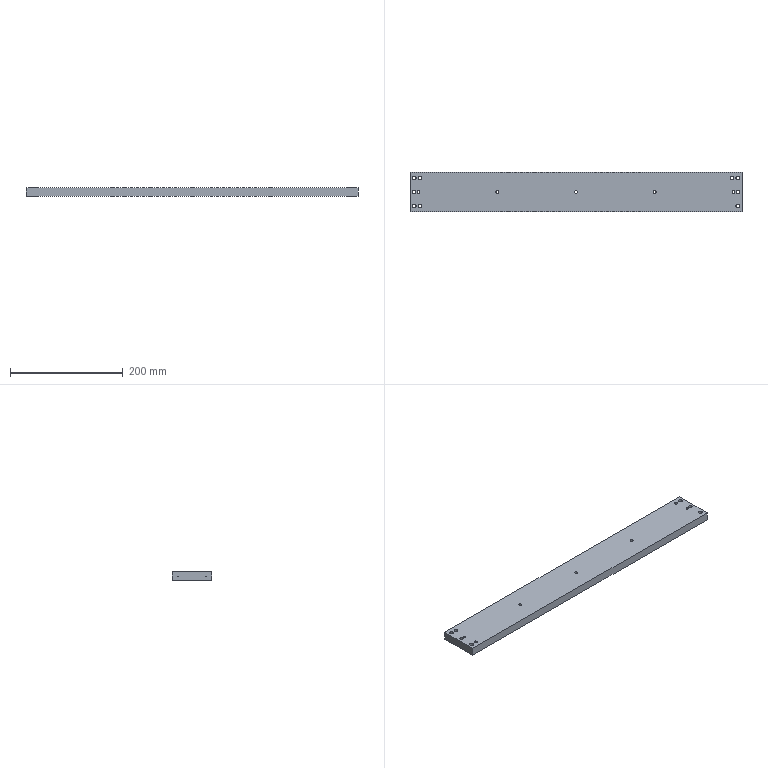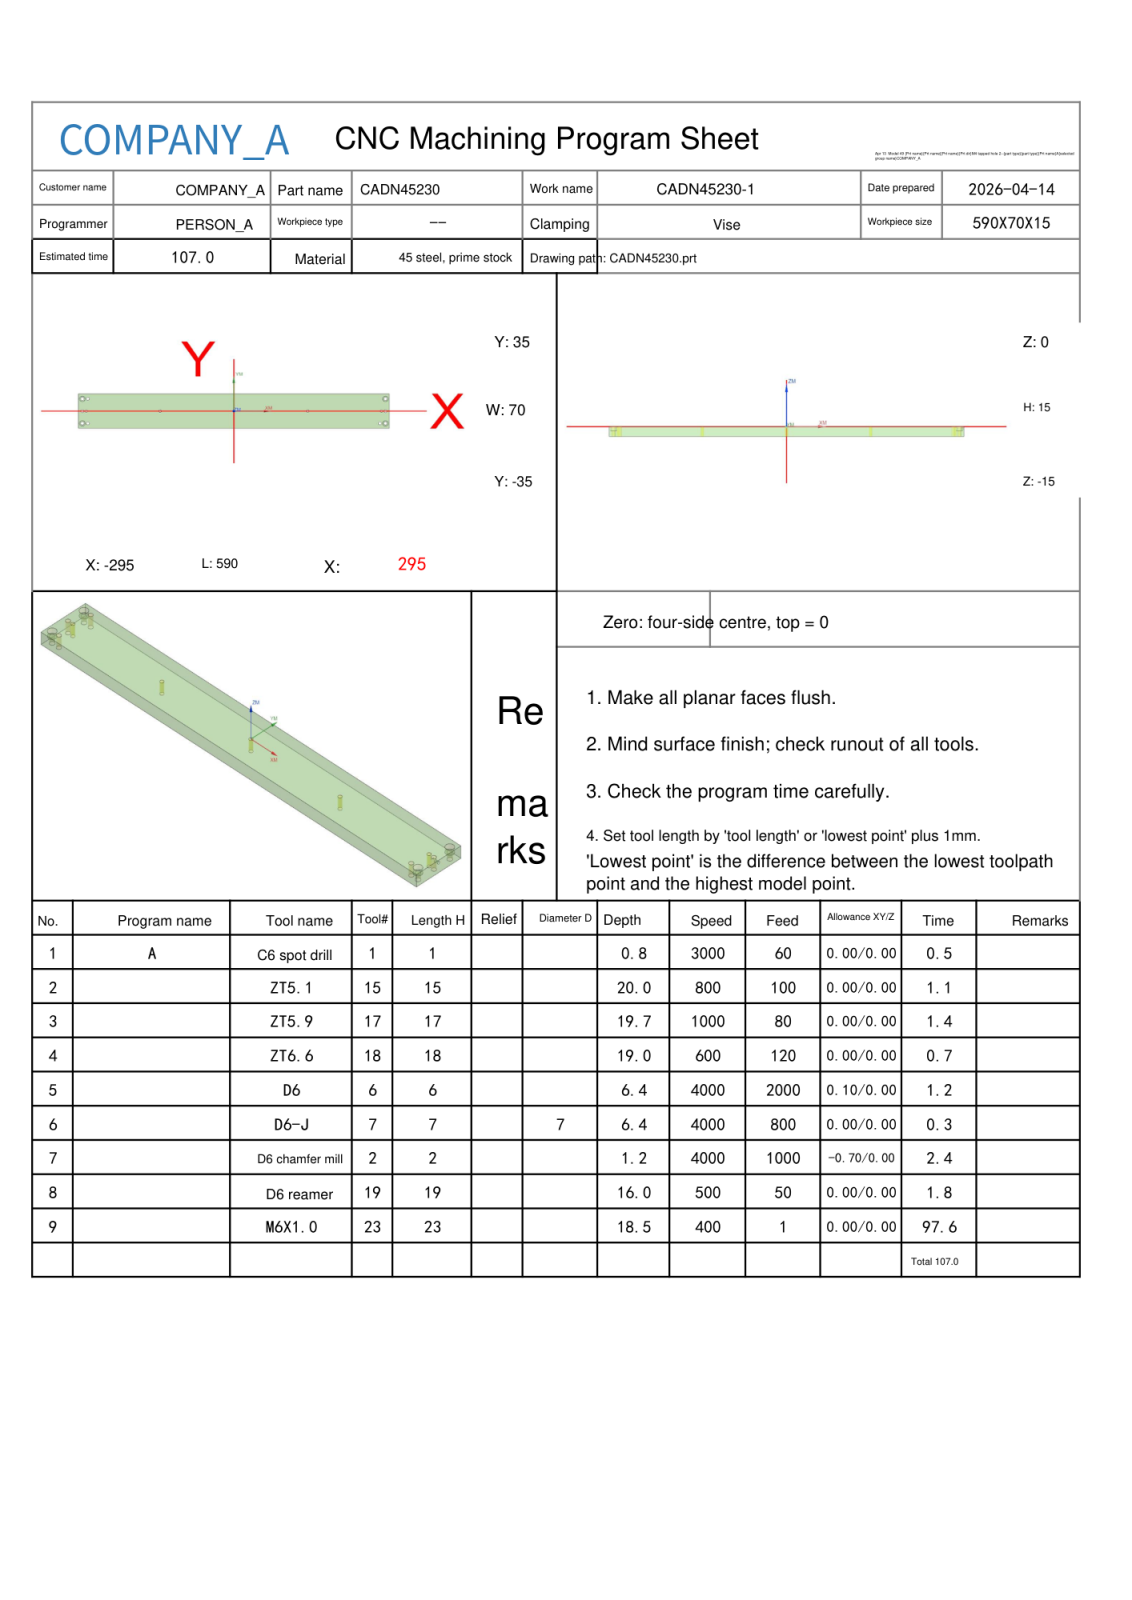NC program | NX | posted by the shop | part box 590 x 70 x 15 mm
Whole program:
%
O0001
(Machine time: 201.23 MIN)
(===Total Tool:9===)
(T1=C6 spot drill   D=6.   R=0.   D-  H01 Z=-0.8  )
(T15=ZT5.1  D=5.1  DR_a=118 D-  H15 Z=-20.  )
(T17=ZT5.9  D=5.9  DR_a=120 D-  H17 Z=-19.7 )
(T18=ZT6.6  D=6.6  DR_a=118 D-  H18 Z=-18.98)
(T6=D6      D=6.   R=0.   D-  H06 Z=-6.4  )
(T7=D6-J    D=6.   R=0.   D7  H07 Z=-6.4  )
(T2=D6 chamfer mill   D=6.   R=0.   D-  H02 Z=-1.2  )
(T19=D6 reamer   D=6.   DR_a=180 D-  H19 Z=-16.  )
(T23=M6X1.0 D=5.   DR_a=180 D-  H23 Z=-18.5 )
G80 G90 G17 G49 G40
G91 G28 Z0
M01
N1 T01 M06
(C6 spot drill  D=6. R=0. H=01 ce=0.00 di=0.00)
G00 G90 G54 X287.5 Y25. M03 S3000
G43 H01 Z20.
M08
G98 G81 X287.5 Y25. Z-.8 R1. F60.
X280. Y0.0
X287.5
Y-25.
X277.
X140. Y0.0
X0.0
X-140.
X-277. Y-25.
X-287.5
Y0.0
X-280.
X-277. Y25.
X-287.5
G80
G00 Z20.
G91 G28 Z0.0
M05
M09
G91 G28 Z0.0
M01
N2 T15 M06
(ZT5.1 D=5.1 DR_a=118 H=15)
G00 G90 G54 X-280. Y0.0 M03 S800
G43 H15 Z20.
M08
G98 G83 X-280. Y0.0 Z-20. R1. F100. Q2.
X-140.
X0.0
X140.
X280.
G80
G00 Z20.
G91 G28 Z0.0
M05
M09
G91 G28 Z0.0
M01
N3 T17 M06
(ZT5.9 D=5.9 DR_a=120 H=17)
G00 G90 G54 X-277. Y25. M03 S1000
G43 H17 Z20.
M08
G98 G83 X-277. Y25. Z-19.703 R1. F80. Q1.
X-287.5 Y0.0
X-277. Y-25.
X277.
X287.5 Y0.0
G80
G00 Z20.
G91 G28 Z0.0
M05
M09
G91 G28 Z0.0
M01
N4 T18 M06
(ZT6.6 D=6.6 DR_a=118 H=18)
G00 G90 G54 X-287.5 Y-25. M03 S600
G43 H18 Z20.
M08
G98 G83 X-287.5 Y-25. Z-18.983 R1. F120. Q2.
Y25.
X287.5
Y-25.
G80
G00 Z20.
G91 G28 Z0.0
M05
M09
G91 G28 Z0.0
M01
N5 T06 M06
(D6  D=6. R=0. H=06 ce=0.10 di=0.00)
G00 G90 G54 X-287.5 Y-25. M03 S4000
G43 H06 Z20.
M08
Z.5
G03 X-286.3 Y-26.2 I1.2 J0.0 F2000.
X-285.1 Y-25. I0.0 J1.2
X-285.1 Y-25. Z.3 I-2.4 J0.0
X-285.1 Y-25. Z.1 I-2.4 J0.0
X-285.1 Y-25. Z-.1 I-2.4 J0.0
X-285.1 Y-25. Z-.3 I-2.4 J0.0
X-285.1 Y-25. Z-.5 I-2.4 J0.0
X-285.1 Y-25. Z-.7 I-2.4 J0.0
X-285.1 Y-25. Z-.9 I-2.4 J0.0
X-285.1 Y-25. Z-1.1 I-2.4 J0.0
X-285.1 Y-25. Z-1.3 I-2.4 J0.0
X-285.1 Y-25. Z-1.5 I-2.4 J0.0
X-285.1 Y-25. Z-1.7 I-2.4 J0.0
X-285.1 Y-25. Z-1.9 I-2.4 J0.0
X-285.1 Y-25. Z-2.1 I-2.4 J0.0
X-285.1 Y-25. Z-2.3 I-2.4 J0.0
X-285.1 Y-25. Z-2.5 I-2.4 J0.0
X-285.1 Y-25. Z-2.7 I-2.4 J0.0
X-285.1 Y-25. Z-2.9 I-2.4 J0.0
X-285.1 Y-25. Z-3.1 I-2.4 J0.0
X-285.1 Y-25. Z-3.3 I-2.4 J0.0
X-285.1 Y-25. Z-3.5 I-2.4 J0.0
X-285.1 Y-25. Z-3.7 I-2.4 J0.0
X-285.1 Y-25. Z-3.9 I-2.4 J0.0
X-285.1 Y-25. Z-4.1 I-2.4 J0.0
X-285.1 Y-25. Z-4.3 I-2.4 J0.0
X-285.1 Y-25. Z-4.5 I-2.4 J0.0
X-285.1 Y-25. Z-4.7 I-2.4 J0.0
X-285.1 Y-25. Z-4.9 I-2.4 J0.0
X-285.1 Y-25. Z-5.1 I-2.4 J0.0
X-285.1 Y-25. Z-5.3 I-2.4 J0.0
X-285.1 Y-25. Z-5.5 I-2.4 J0.0
X-285.1 Y-25. Z-5.7 I-2.4 J0.0
X-285.1 Y-25. Z-5.9 I-2.4 J0.0
X-285.1 Y-25. Z-6.1 I-2.4 J0.0
X-285.1 Y-25. Z-6.3 I-2.4 J0.0
X-289.9 Y-25. Z-6.4 I-2.4 J0.0
X-287.5 Y-27.4 I2.4 J0.0
X-285.1 Y-25. I0.0 J2.4
X-287.5 Y-22.6 I-2.4 J0.0
X-289.9 Y-25. I0.0 J-2.4
X-288.7 Y-26.2 I1.2 J0.0
X-287.5 Y-25. I0.0 J1.2
G00 Z20.
Y25.
Z.5
G03 X-286.3 Y23.8 I1.2 J0.0
X-285.1 Y25. I0.0 J1.2
X-285.1 Y25. Z.3 I-2.4 J0.0
X-285.1 Y25. Z.1 I-2.4 J0.0
X-285.1 Y25. Z-.1 I-2.4 J0.0
X-285.1 Y25. Z-.3 I-2.4 J0.0
X-285.1 Y25. Z-.5 I-2.4 J0.0
X-285.1 Y25. Z-.7 I-2.4 J0.0
X-285.1 Y25. Z-.9 I-2.4 J0.0
X-285.1 Y25. Z-1.1 I-2.4 J0.0
X-285.1 Y25. Z-1.3 I-2.4 J0.0
X-285.1 Y25. Z-1.5 I-2.4 J0.0
X-285.1 Y25. Z-1.7 I-2.4 J0.0
X-285.1 Y25. Z-1.9 I-2.4 J0.0
X-285.1 Y25. Z-2.1 I-2.4 J0.0
X-285.1 Y25. Z-2.3 I-2.4 J0.0
X-285.1 Y25. Z-2.5 I-2.4 J0.0
X-285.1 Y25. Z-2.7 I-2.4 J0.0
X-285.1 Y25. Z-2.9 I-2.4 J0.0
X-285.1 Y25. Z-3.1 I-2.4 J0.0
X-285.1 Y25. Z-3.3 I-2.4 J0.0
X-285.1 Y25. Z-3.5 I-2.4 J0.0
X-285.1 Y25. Z-3.7 I-2.4 J0.0
X-285.1 Y25. Z-3.9 I-2.4 J0.0
X-285.1 Y25. Z-4.1 I-2.4 J0.0
X-285.1 Y25. Z-4.3 I-2.4 J0.0
X-285.1 Y25. Z-4.5 I-2.4 J0.0
X-285.1 Y25. Z-4.7 I-2.4 J0.0
X-285.1 Y25. Z-4.9 I-2.4 J0.0
X-285.1 Y25. Z-5.1 I-2.4 J0.0
X-285.1 Y25. Z-5.3 I-2.4 J0.0
X-285.1 Y25. Z-5.5 I-2.4 J0.0
X-285.1 Y25. Z-5.7 I-2.4 J0.0
X-285.1 Y25. Z-5.9 I-2.4 J0.0
X-285.1 Y25. Z-6.1 I-2.4 J0.0
X-285.1 Y25. Z-6.3 I-2.4 J0.0
X-289.9 Y25. Z-6.4 I-2.4 J0.0
X-287.5 Y22.6 I2.4 J0.0
X-285.1 Y25. I0.0 J2.4
X-287.5 Y27.4 I-2.4 J0.0
X-289.9 Y25. I0.0 J-2.4
X-288.7 Y23.8 I1.2 J0.0
X-287.5 Y25. I0.0 J1.2
G00 Z20.
X287.5
Z.5
G03 X288.7 Y23.8 I1.2 J0.0
X289.9 Y25. I0.0 J1.2
X289.9 Y25. Z.3 I-2.4 J0.0
X289.9 Y25. Z.1 I-2.4 J0.0
X289.9 Y25. Z-.1 I-2.4 J0.0
X289.9 Y25. Z-.3 I-2.4 J0.0
X289.9 Y25. Z-.5 I-2.4 J0.0
X289.9 Y25. Z-.7 I-2.4 J0.0
X289.9 Y25. Z-.9 I-2.4 J0.0
X289.9 Y25. Z-1.1 I-2.4 J0.0
X289.9 Y25. Z-1.3 I-2.4 J0.0
X289.9 Y25. Z-1.5 I-2.4 J0.0
X289.9 Y25. Z-1.7 I-2.4 J0.0
X289.9 Y25. Z-1.9 I-2.4 J0.0
X289.9 Y25. Z-2.1 I-2.4 J0.0
X289.9 Y25. Z-2.3 I-2.4 J0.0
X289.9 Y25. Z-2.5 I-2.4 J0.0
X289.9 Y25. Z-2.7 I-2.4 J0.0
X289.9 Y25. Z-2.9 I-2.4 J0.0
X289.9 Y25. Z-3.1 I-2.4 J0.0
X289.9 Y25. Z-3.3 I-2.4 J0.0
X289.9 Y25. Z-3.5 I-2.4 J0.0
X289.9 Y25. Z-3.7 I-2.4 J0.0
X289.9 Y25. Z-3.9 I-2.4 J0.0
X289.9 Y25. Z-4.1 I-2.4 J0.0
X289.9 Y25. Z-4.3 I-2.4 J0.0
X289.9 Y25. Z-4.5 I-2.4 J0.0
X289.9 Y25. Z-4.7 I-2.4 J0.0
X289.9 Y25. Z-4.9 I-2.4 J0.0
X289.9 Y25. Z-5.1 I-2.4 J0.0
X289.9 Y25. Z-5.3 I-2.4 J0.0
X289.9 Y25. Z-5.5 I-2.4 J0.0
X289.9 Y25. Z-5.7 I-2.4 J0.0
X289.9 Y25. Z-5.9 I-2.4 J0.0
X289.9 Y25. Z-6.1 I-2.4 J0.0
X289.9 Y25. Z-6.3 I-2.4 J0.0
X285.1 Y25. Z-6.4 I-2.4 J0.0
X287.5 Y22.6 I2.4 J0.0
X289.9 Y25. I0.0 J2.4
X287.5 Y27.4 I-2.4 J0.0
X285.1 Y25. I0.0 J-2.4
X286.3 Y23.8 I1.2 J0.0
X287.5 Y25. I0.0 J1.2
G00 Z20.
Y-25.
Z.5
G03 X288.7 Y-26.2 I1.2 J0.0
X289.9 Y-25. I0.0 J1.2
X289.9 Y-25. Z.3 I-2.4 J0.0
X289.9 Y-25. Z.1 I-2.4 J0.0
X289.9 Y-25. Z-.1 I-2.4 J0.0
X289.9 Y-25. Z-.3 I-2.4 J0.0
X289.9 Y-25. Z-.5 I-2.4 J0.0
X289.9 Y-25. Z-.7 I-2.4 J0.0
X289.9 Y-25. Z-.9 I-2.4 J0.0
X289.9 Y-25. Z-1.1 I-2.4 J0.0
X289.9 Y-25. Z-1.3 I-2.4 J0.0
X289.9 Y-25. Z-1.5 I-2.4 J0.0
X289.9 Y-25. Z-1.7 I-2.4 J0.0
X289.9 Y-25. Z-1.9 I-2.4 J0.0
X289.9 Y-25. Z-2.1 I-2.4 J0.0
X289.9 Y-25. Z-2.3 I-2.4 J0.0
X289.9 Y-25. Z-2.5 I-2.4 J0.0
X289.9 Y-25. Z-2.7 I-2.4 J0.0
X289.9 Y-25. Z-2.9 I-2.4 J0.0
X289.9 Y-25. Z-3.1 I-2.4 J0.0
X289.9 Y-25. Z-3.3 I-2.4 J0.0
X289.9 Y-25. Z-3.5 I-2.4 J0.0
X289.9 Y-25. Z-3.7 I-2.4 J0.0
X289.9 Y-25. Z-3.9 I-2.4 J0.0
X289.9 Y-25. Z-4.1 I-2.4 J0.0
X289.9 Y-25. Z-4.3 I-2.4 J0.0
X289.9 Y-25. Z-4.5 I-2.4 J0.0
X289.9 Y-25. Z-4.7 I-2.4 J0.0
X289.9 Y-25. Z-4.9 I-2.4 J0.0
X289.9 Y-25. Z-5.1 I-2.4 J0.0
X289.9 Y-25. Z-5.3 I-2.4 J0.0
X289.9 Y-25. Z-5.5 I-2.4 J0.0
X289.9 Y-25. Z-5.7 I-2.4 J0.0
X289.9 Y-25. Z-5.9 I-2.4 J0.0
X289.9 Y-25. Z-6.1 I-2.4 J0.0
X289.9 Y-25. Z-6.3 I-2.4 J0.0
X285.1 Y-25. Z-6.4 I-2.4 J0.0
X287.5 Y-27.4 I2.4 J0.0
X289.9 Y-25. I0.0 J2.4
X287.5 Y-22.6 I-2.4 J0.0
X285.1 Y-25. I0.0 J-2.4
X286.3 Y-26.2 I1.2 J0.0
X287.5 Y-25. I0.0 J1.2
G00 Z20.
G91 G28 Z0.0
M05
M09
G91 G28 Z0.0
M01
N6 T07 M06
(D6-J  D=6. R=0. H=07 ce=0.00 di=0.00)
G00 G90 G54 X-287.5 Y-25. M03 S4000
G43 H07 Z20.
M08
Z0.0
G41 D07
G01 X-287.468 Y-25.197 F800.
G03 X-286.242 Y-26.242 I1.226 J.197
X-285. Y-25. I0.0 J1.242
X-285. Y-25. Z-5. I-2.5 J0.0
X-287.968 Y-22.544 Z-6.4 I-2.5 J0.0
X-290. Y-25. I.468 J-2.456
X-287.5 Y-27.5 I2.5 J0.0
X-285. Y-25. I0.0 J2.5
X-287.5 Y-22.5 I-2.5 J0.0
X-287.968 Y-22.544 I0.0 J-2.5
X-288.978 Y-23.764 I.233 J-1.22
X-287.736 Y-25.006 I1.242 J0.0
G01 X-287.7
G40 X-287.5 Y-25.
G00 Z20.
Y25.
Z0.0
G41 D07
G01 X-287.468 Y24.803
G03 X-286.242 Y23.758 I1.226 J.197
X-285. Y25. I0.0 J1.242
X-285. Y25. Z-5. I-2.5 J0.0
X-287.968 Y27.456 Z-6.4 I-2.5 J0.0
X-290. Y25. I.468 J-2.456
X-287.5 Y22.5 I2.5 J0.0
X-285. Y25. I0.0 J2.5
X-287.5 Y27.5 I-2.5 J0.0
X-287.968 Y27.456 I0.0 J-2.5
X-288.978 Y26.236 I.233 J-1.22
X-287.736 Y24.994 I1.242 J0.0
G01 X-287.7
G40 X-287.5 Y25.
G00 Z20.
X287.5
Z0.0
G41 D07
G01 X287.532 Y24.803
G03 X288.758 Y23.758 I1.226 J.197
X290. Y25. I0.0 J1.242
X290. Y25. Z-5. I-2.5 J0.0
X287.032 Y27.456 Z-6.4 I-2.5 J0.0
X285. Y25. I.468 J-2.456
X287.5 Y22.5 I2.5 J0.0
X290. Y25. I0.0 J2.5
X287.5 Y27.5 I-2.5 J0.0
X287.032 Y27.456 I0.0 J-2.5
X286.022 Y26.236 I.233 J-1.22
X287.264 Y24.994 I1.242 J0.0
G01 X287.3
G40 X287.5 Y25.
G00 Z20.
Y-25.
Z0.0
G41 D07
G01 X287.532 Y-25.197
G03 X288.758 Y-26.242 I1.226 J.197
X290. Y-25. I0.0 J1.242
X290. Y-25. Z-5. I-2.5 J0.0
X287.032 Y-22.544 Z-6.4 I-2.5 J0.0
X285. Y-25. I.468 J-2.456
X287.5 Y-27.5 I2.5 J0.0
X290. Y-25. I0.0 J2.5
X287.5 Y-22.5 I-2.5 J0.0
X287.032 Y-22.544 I0.0 J-2.5
X286.022 Y-23.764 I.233 J-1.22
X287.264 Y-25.006 I1.242 J0.0
G01 X287.3
G40 X287.5 Y-25.
G00 Z20.
G91 G28 Z0.0
M05
M09
G91 G28 Z0.0
M01
N7 T02 M06
(D6 chamfer mill  D=6. R=0. H=02 ce=-0.30 di=0.00)
G00 G90 G54 X-276.388 Y23.853 M03 S4000
G43 H02 Z20.
M08
Z-.5
G01 Z-1. F400.
X-276.2 Y23.5
G03 X-274.7 Y25. I0.0 J1.5
X-277. Y27.3 I-2.3 J0.0
X-279.3 Y25. I0.0 J-2.3
X-277. Y22.7 I2.3 J0.0
X-274.7 Y25. I0.0 J2.3
X-276.2 Y26.5 I-1.5 J0.0
G01 X-276.388 Y26.147
Z-.5
G00 Z20.
X-286.888 Y-1.147
Z-.5
G01 Z-1.
X-286.7 Y-1.5
G03 X-285.2 Y0.0 I0.0 J1.5
X-287.5 Y2.3 I-2.3 J0.0
X-289.8 Y0.0 I0.0 J-2.3
X-287.5 Y-2.3 I2.3 J0.0
X-285.2 Y0.0 I0.0 J2.3
X-286.7 Y1.5 I-1.5 J0.0
G01 X-286.888 Y1.147
Z-.5
G00 Z20.
X-276.388 Y-26.147
Z-.5
G01 Z-1.
X-276.2 Y-26.5
G03 X-274.7 Y-25. I0.0 J1.5
X-277. Y-22.7 I-2.3 J0.0
X-279.3 Y-25. I0.0 J-2.3
X-277. Y-27.3 I2.3 J0.0
X-274.7 Y-25. I0.0 J2.3
X-276.2 Y-23.5 I-1.5 J0.0
G01 X-276.388 Y-23.853
Z-.5
G00 Z20.
X277.612 Y-26.147
Z-.5
G01 Z-1.
X277.8 Y-26.5
G03 X279.3 Y-25. I0.0 J1.5
X277. Y-22.7 I-2.3 J0.0
X274.7 Y-25. I0.0 J-2.3
X277. Y-27.3 I2.3 J0.0
X279.3 Y-25. I0.0 J2.3
X277.8 Y-23.5 I-1.5 J0.0
G01 X277.612 Y-23.853
Z-.5
G00 Z20.
X288.112 Y-1.147
Z-.5
G01 Z-1.
X288.3 Y-1.5
G03 X289.8 Y0.0 I0.0 J1.5
X287.5 Y2.3 I-2.3 J0.0
X285.2 Y0.0 I0.0 J-2.3
X287.5 Y-2.3 I2.3 J0.0
X289.8 Y0.0 I0.0 J2.3
X288.3 Y1.5 I-1.5 J0.0
G01 X288.112 Y1.147
Z-.5
G00 Z20.
G00 G90 X289.509 Y29.357 M03 S4000
Z20.
Z2.5
G01 X289.334 Y29.439 Z2.43 F800.
X288.899 Y29.595 Z2.261
X288.45 Y29.708 Z2.093
X287.993 Y29.778 Z1.925
X287.531 Y29.803 Z1.756
X287.069 Y29.784 Z1.588
X286.61 Y29.72 Z1.419
X286.16 Y29.612 Z1.251
X285.723 Y29.462 Z1.083
X285.302 Y29.27 Z.914
X284.901 Y29.039 Z.746
X284.524 Y28.77 Z.577
X284.175 Y28.466 Z.409
X283.857 Y28.13 Z.241
X283.573 Y27.765 Z.072
X283.325 Y27.375 Z-.096
X283.116 Y26.962 Z-.265
X282.948 Y26.531 Z-.433
X282.821 Y26.086 Z-.601
X282.739 Y25.631 Z-.77
X282.7 Y25.17 Z-.938
Y25. Z-1.
G03 X287.5 Y20.2 I4.8 J0.0
X292.3 Y25. I0.0 J4.8
X287.5 Y29.8 I-4.8 J0.0
X282.7 Y25. I0.0 J-4.8
X282.726 Y24.501 I4.8 J0.0
G01 Z1.5
G00 Z20.
X289.509 Y-20.643
Z2.5
G01 X289.334 Y-20.561 Z2.43
X288.899 Y-20.405 Z2.261
X288.45 Y-20.292 Z2.093
X287.993 Y-20.222 Z1.925
X287.531 Y-20.197 Z1.756
X287.069 Y-20.216 Z1.588
X286.61 Y-20.28 Z1.419
X286.16 Y-20.388 Z1.251
X285.723 Y-20.538 Z1.083
X285.302 Y-20.73 Z.914
X284.901 Y-20.961 Z.746
X284.524 Y-21.23 Z.577
X284.175 Y-21.534 Z.409
X283.857 Y-21.87 Z.241
X283.573 Y-22.235 Z.072
X283.325 Y-22.625 Z-.096
X283.116 Y-23.038 Z-.265
X282.948 Y-23.469 Z-.433
X282.821 Y-23.914 Z-.601
X282.739 Y-24.369 Z-.77
X282.7 Y-24.83 Z-.938
Y-25. Z-1.
G03 X287.5 Y-29.8 I4.8 J0.0
X292.3 Y-25. I0.0 J4.8
X287.5 Y-20.2 I-4.8 J0.0
X282.7 Y-25. I0.0 J-4.8
X282.726 Y-25.499 I4.8 J0.0
G01 Z1.5
G00 Z20.
X-285.491 Y-20.643
Z2.5
G01 X-285.666 Y-20.561 Z2.43
X-286.101 Y-20.405 Z2.261
X-286.55 Y-20.292 Z2.093
X-287.007 Y-20.222 Z1.925
X-287.469 Y-20.197 Z1.756
X-287.931 Y-20.216 Z1.588
X-288.39 Y-20.28 Z1.419
X-288.84 Y-20.388 Z1.251
X-289.277 Y-20.538 Z1.083
X-289.698 Y-20.73 Z.914
X-290.099 Y-20.961 Z.746
X-290.476 Y-21.23 Z.577
X-290.825 Y-21.534 Z.409
X-291.143 Y-21.87 Z.241
X-291.427 Y-22.235 Z.072
X-291.675 Y-22.625 Z-.096
X-291.884 Y-23.038 Z-.265
X-292.052 Y-23.469 Z-.433
X-292.179 Y-23.914 Z-.601
X-292.261 Y-24.369 Z-.77
X-292.3 Y-24.83 Z-.938
Y-25. Z-1.
G03 X-287.5 Y-29.8 I4.8 J0.0
X-282.7 Y-25. I0.0 J4.8
X-287.5 Y-20.2 I-4.8 J0.0
X-292.3 Y-25. I0.0 J-4.8
X-292.274 Y-25.499 I4.8 J0.0
G01 Z1.5
G00 Z20.
X-285.491 Y29.357
Z2.5
G01 X-285.666 Y29.439 Z2.43
X-286.101 Y29.595 Z2.261
X-286.55 Y29.708 Z2.093
X-287.007 Y29.778 Z1.925
X-287.469 Y29.803 Z1.756
X-287.931 Y29.784 Z1.588
X-288.39 Y29.72 Z1.419
X-288.84 Y29.612 Z1.251
X-289.277 Y29.462 Z1.083
X-289.698 Y29.27 Z.914
X-290.099 Y29.039 Z.746
X-290.476 Y28.77 Z.577
X-290.825 Y28.466 Z.409
X-291.143 Y28.13 Z.241
X-291.427 Y27.765 Z.072
X-291.675 Y27.375 Z-.096
X-291.884 Y26.962 Z-.265
X-292.052 Y26.531 Z-.433
X-292.179 Y26.086 Z-.601
X-292.261 Y25.631 Z-.77
X-292.3 Y25.17 Z-.938
Y25. Z-1.
G03 X-287.5 Y20.2 I4.8 J0.0
X-282.7 Y25. I0.0 J4.8
X-287.5 Y29.8 I-4.8 J0.0
X-292.3 Y25. I0.0 J-4.8
X-292.274 Y24.501 I4.8 J0.0
G01 Z1.5
G00 Z20.
G00 G90 X-279.591 Y-1.021 M03 S4000
Z20.
Z-.6
G01 Z-1.1 F300.
X-279.4 Y-1.5
G03 X-277.9 Y0.0 I0.0 J1.5
X-280. Y2.1 I-2.1 J0.0
X-282.1 Y0.0 I0.0 J-2.1
X-280. Y-2.1 I2.1 J0.0
X-277.9 Y0.0 I0.0 J2.1
X-279.4 Y1.5 I-1.5 J0.0
G01 X-279.591 Y1.021
Z-.6
G00 Z20.
X-139.591 Y-1.021
Z-.6
G01 Z-1.1
X-139.4 Y-1.5
G03 X-137.9 Y0.0 I0.0 J1.5
X-140. Y2.1 I-2.1 J0.0
X-142.1 Y0.0 I0.0 J-2.1
X-140. Y-2.1 I2.1 J0.0
X-137.9 Y0.0 I0.0 J2.1
X-139.4 Y1.5 I-1.5 J0.0
G01 X-139.591 Y1.021
Z-.6
G00 Z20.
X.409 Y-1.021
Z-.6
G01 Z-1.1
X.6 Y-1.5
G03 X2.1 Y0.0 I0.0 J1.5
X0.0 Y2.1 I-2.1 J0.0
X-2.1 Y0.0 I0.0 J-2.1
X0.0 Y-2.1 I2.1 J0.0
X2.1 Y0.0 I0.0 J2.1
X.6 Y1.5 I-1.5 J0.0
G01 X.409 Y1.021
Z-.6
G00 Z20.
X140.409 Y-1.021
Z-.6
G01 Z-1.1
X140.6 Y-1.5
G03 X142.1 Y0.0 I0.0 J1.5
X140. Y2.1 I-2.1 J0.0
X137.9 Y0.0 I0.0 J-2.1
X140. Y-2.1 I2.1 J0.0
X142.1 Y0.0 I0.0 J2.1
X140.6 Y1.5 I-1.5 J0.0
G01 X140.409 Y1.021
Z-.6
G00 Z20.
X280.409 Y-1.021
Z-.6
G01 Z-1.1
X280.6 Y-1.5
G03 X282.1 Y0.0 I0.0 J1.5
X280. Y2.1 I-2.1 J0.0
X277.9 Y0.0 I0.0 J-2.1
X280. Y-2.1 I2.1 J0.0
X282.1 Y0.0 I0.0 J2.1
X280.6 Y1.5 I-1.5 J0.0
G01 X280.409 Y1.021
Z-.6
G00 Z20.
G00 G90 X-295.9 Y26.422 M03 S4000
Z20.
Z2.5
G01 Y34.7 Z-.513 F1000.
Y34.785 Z-.544
X-295.866 Y34.997 Z-.622
X-295.794 Y35.199 Z-.7
X-295.688 Y35.386 Z-.778
X-295.551 Y35.551 Z-.857
X-295.386 Y35.688 Z-.935
X-295.199 Y35.794 Z-1.013
X-294.997 Y35.866 Z-1.091
X-294.785 Y35.9 Z-1.169
X-294.7 Z-1.2
X294.7
G02 X295.9 Y34.7 I0.0 J-1.2
G01 Y-34.7
G02 X294.7 Y-35.9 I-1.2 J0.0
G01 X-294.7
G02 X-295.9 Y-34.7 I0.0 J1.2
G01 Y34.7
G02 X-294.7 Y35.9 I1.2 J0.0
G01 X-294.2
Z1.3
G00 Z20.
G91 G28 Z0.0
M05
M09
G91 G28 Z0.0
M01
N8 T19 M06
(D6 reamer D=6. DR_a=180 H=19)
G00 G90 G54 X-277. Y25. M03 S500
G43 H19 Z20.
M08
G98 G81 X-277. Y25. Z-16. R1. F50.
X-287.5 Y0.0
X-277. Y-25.
X277.
X287.5 Y0.0
G80
G00 Z20.
G91 G28 Z0.0
M05
M09
G91 G28 Z0.0
M01
N9 T23 M06
(M6X1.0 D=5. DR_a=180 H=23)
G00 G90 G54 X-280. Y0.0 M03 S400
G43 H23 Z20.
M08
G95
G98 G84 X-280. Y0.0 Z-18.5 R1. F1. Q2.
X-140.
X0.0
X140.
X280.
G80
G94
G00 Z20.
M05
M09
G91 G28 Z0.0
G91 G28 Y0.0
M30
%